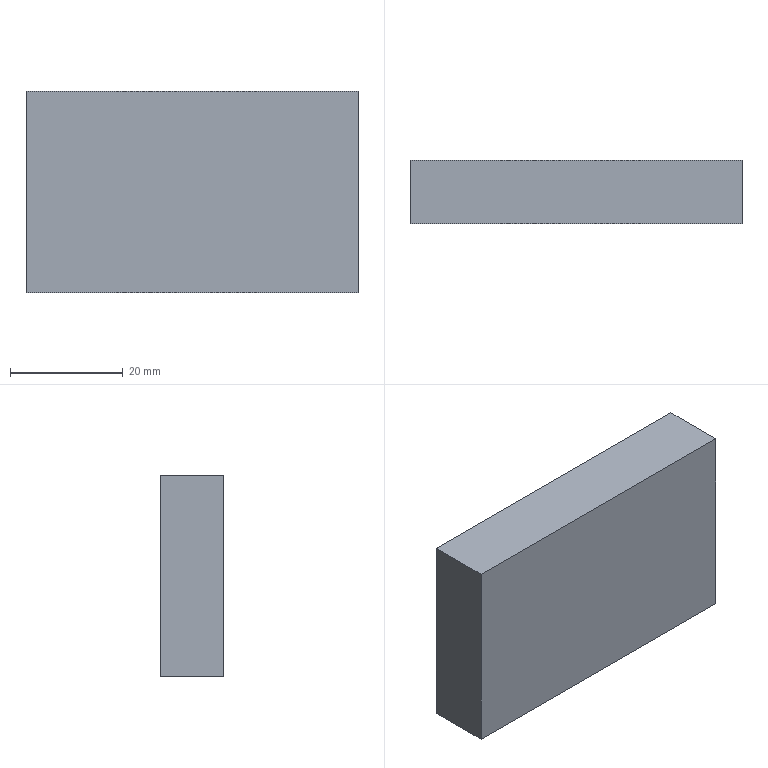Part | STEP file | 1 solid | 6 faces | box 58.8 x 11.27 x 35.77 mm | volume 23704 mm3 | plane 6
STEP:
#1=CARTESIAN_POINT('',(0.,0.,0.));
#2=DIRECTION('',(0.,0.,1.));
#3=DIRECTION('',(1.,0.,0.));
#4=AXIS2_PLACEMENT_3D('',#1,#2,#3);
#5=CARTESIAN_POINT('',(979.439,-73.009,179.647));
#6=VERTEX_POINT('',#5);
#7=CARTESIAN_POINT('',(920.639,-73.009,179.647));
#8=VERTEX_POINT('',#7);
#9=CARTESIAN_POINT('',(979.439,-73.009,179.647));
#10=DIRECTION('',(-1.,0.,0.));
#11=VECTOR('',#10,1.);
#12=LINE('',#9,#11);
#13=CARTESIAN_POINT('',(950.039,-67.374,179.647));
#14=DIRECTION('',(0.,0.,1.));
#15=DIRECTION('',(1.,0.,0.));
#16=AXIS2_PLACEMENT_3D('',#13,#14,#15);
#17=PLANE('',#16);
#18=CARTESIAN_POINT('',(29.4,-5.635));
#19=DIRECTION('',(-1.,0.));
#20=VECTOR('',#19,1.);
#21=LINE('',#18,#20);
#22=(GEOMETRIC_REPRESENTATION_CONTEXT(2)PARAMETRIC_REPRESENTATION_CONTEXT()REPRESENTATION_CONTEXT('',''));
#23=DEFINITIONAL_REPRESENTATION('',(#21),#22);
#24=PCURVE('',#17,#23);
#25=CARTESIAN_POINT('',(979.439,-73.009,143.877));
#26=DIRECTION('',(0.,1.,0.));
#27=DIRECTION('',(-1.,0.,0.));
#28=AXIS2_PLACEMENT_3D('',#25,#26,#27);
#29=PLANE('',#28);
#30=CARTESIAN_POINT('',(0.,35.77));
#31=DIRECTION('',(1.,0.));
#32=VECTOR('',#31,1.);
#33=LINE('',#30,#32);
#34=(GEOMETRIC_REPRESENTATION_CONTEXT(2)PARAMETRIC_REPRESENTATION_CONTEXT()REPRESENTATION_CONTEXT('',''));
#35=DEFINITIONAL_REPRESENTATION('',(#33),#34);
#36=PCURVE('',#29,#35);
#37=SURFACE_CURVE('',#12,(#24,#36),.PCURVE_S1.);
#38=EDGE_CURVE('',#6,#8,#37,.T.);
#39=ORIENTED_EDGE('',*,*,#38,.F.);
#40=CARTESIAN_POINT('',(979.439,-61.739,179.647));
#41=VERTEX_POINT('',#40);
#42=CARTESIAN_POINT('',(979.439,-73.009,179.647));
#43=DIRECTION('',(0.,1.,0.));
#44=VECTOR('',#43,1.);
#45=LINE('',#42,#44);
#46=CARTESIAN_POINT('',(29.4,-5.635));
#47=DIRECTION('',(0.,1.));
#48=VECTOR('',#47,1.);
#49=LINE('',#46,#48);
#50=(GEOMETRIC_REPRESENTATION_CONTEXT(2)PARAMETRIC_REPRESENTATION_CONTEXT()REPRESENTATION_CONTEXT('',''));
#51=DEFINITIONAL_REPRESENTATION('',(#49),#50);
#52=PCURVE('',#17,#51);
#53=CARTESIAN_POINT('',(979.439,-73.009,143.877));
#54=DIRECTION('',(1.,0.,0.));
#55=DIRECTION('',(0.,0.,-1.));
#56=AXIS2_PLACEMENT_3D('',#53,#54,#55);
#57=PLANE('',#56);
#58=CARTESIAN_POINT('',(-35.77,0.));
#59=DIRECTION('',(0.,1.));
#60=VECTOR('',#59,1.);
#61=LINE('',#58,#60);
#62=(GEOMETRIC_REPRESENTATION_CONTEXT(2)PARAMETRIC_REPRESENTATION_CONTEXT()REPRESENTATION_CONTEXT('',''));
#63=DEFINITIONAL_REPRESENTATION('',(#61),#62);
#64=PCURVE('',#57,#63);
#65=SURFACE_CURVE('',#45,(#52,#64),.PCURVE_S1.);
#66=EDGE_CURVE('',#6,#41,#65,.T.);
#67=ORIENTED_EDGE('',*,*,#66,.T.);
#68=CARTESIAN_POINT('',(920.639,-61.739,179.647));
#69=VERTEX_POINT('',#68);
#70=CARTESIAN_POINT('',(979.439,-61.739,179.647));
#71=DIRECTION('',(-1.,0.,0.));
#72=VECTOR('',#71,1.);
#73=LINE('',#70,#72);
#74=CARTESIAN_POINT('',(29.4,5.635));
#75=DIRECTION('',(-1.,0.));
#76=VECTOR('',#75,1.);
#77=LINE('',#74,#76);
#78=(GEOMETRIC_REPRESENTATION_CONTEXT(2)PARAMETRIC_REPRESENTATION_CONTEXT()REPRESENTATION_CONTEXT('',''));
#79=DEFINITIONAL_REPRESENTATION('',(#77),#78);
#80=PCURVE('',#17,#79);
#81=CARTESIAN_POINT('',(979.439,-61.739,143.877));
#82=DIRECTION('',(0.,1.,0.));
#83=DIRECTION('',(-1.,0.,0.));
#84=AXIS2_PLACEMENT_3D('',#81,#82,#83);
#85=PLANE('',#84);
#86=CARTESIAN_POINT('',(0.,35.77));
#87=DIRECTION('',(1.,0.));
#88=VECTOR('',#87,1.);
#89=LINE('',#86,#88);
#90=(GEOMETRIC_REPRESENTATION_CONTEXT(2)PARAMETRIC_REPRESENTATION_CONTEXT()REPRESENTATION_CONTEXT('',''));
#91=DEFINITIONAL_REPRESENTATION('',(#89),#90);
#92=PCURVE('',#85,#91);
#93=SURFACE_CURVE('',#73,(#80,#92),.PCURVE_S1.);
#94=EDGE_CURVE('',#41,#69,#93,.T.);
#95=ORIENTED_EDGE('',*,*,#94,.T.);
#96=CARTESIAN_POINT('',(920.639,-61.739,179.647));
#97=DIRECTION('',(0.,-1.,0.));
#98=VECTOR('',#97,1.);
#99=LINE('',#96,#98);
#100=CARTESIAN_POINT('',(-29.4,5.635));
#101=DIRECTION('',(0.,-1.));
#102=VECTOR('',#101,1.);
#103=LINE('',#100,#102);
#104=(GEOMETRIC_REPRESENTATION_CONTEXT(2)PARAMETRIC_REPRESENTATION_CONTEXT()REPRESENTATION_CONTEXT('',''));
#105=DEFINITIONAL_REPRESENTATION('',(#103),#104);
#106=PCURVE('',#17,#105);
#107=CARTESIAN_POINT('',(920.639,-61.739,143.877));
#108=DIRECTION('',(-1.,0.,0.));
#109=DIRECTION('',(0.,-1.,0.));
#110=AXIS2_PLACEMENT_3D('',#107,#108,#109);
#111=PLANE('',#110);
#112=CARTESIAN_POINT('',(0.,35.77));
#113=DIRECTION('',(1.,0.));
#114=VECTOR('',#113,1.);
#115=LINE('',#112,#114);
#116=(GEOMETRIC_REPRESENTATION_CONTEXT(2)PARAMETRIC_REPRESENTATION_CONTEXT()REPRESENTATION_CONTEXT('',''));
#117=DEFINITIONAL_REPRESENTATION('',(#115),#116);
#118=PCURVE('',#111,#117);
#119=SURFACE_CURVE('',#99,(#106,#118),.PCURVE_S1.);
#120=EDGE_CURVE('',#69,#8,#119,.T.);
#121=ORIENTED_EDGE('',*,*,#120,.T.);
#122=EDGE_LOOP('',(#39,#67,#95,#121));
#123=FACE_BOUND('',#122,.T.);
#124=ADVANCED_FACE('',(#123),#17,.T.);
#125=CARTESIAN_POINT('',(979.439,-73.009,143.877));
#126=VERTEX_POINT('',#125);
#127=CARTESIAN_POINT('',(920.639,-73.009,143.877));
#128=VERTEX_POINT('',#127);
#129=CARTESIAN_POINT('',(979.439,-73.009,143.877));
#130=DIRECTION('',(-1.,0.,0.));
#131=VECTOR('',#130,1.);
#132=LINE('',#129,#131);
#133=CARTESIAN_POINT('',(950.039,-67.374,143.877));
#134=DIRECTION('',(0.,0.,1.));
#135=DIRECTION('',(1.,0.,0.));
#136=AXIS2_PLACEMENT_3D('',#133,#134,#135);
#137=PLANE('',#136);
#138=CARTESIAN_POINT('',(29.4,-5.635));
#139=DIRECTION('',(-1.,0.));
#140=VECTOR('',#139,1.);
#141=LINE('',#138,#140);
#142=(GEOMETRIC_REPRESENTATION_CONTEXT(2)PARAMETRIC_REPRESENTATION_CONTEXT()REPRESENTATION_CONTEXT('',''));
#143=DEFINITIONAL_REPRESENTATION('',(#141),#142);
#144=PCURVE('',#137,#143);
#145=CARTESIAN_POINT('',(0.,0.));
#146=DIRECTION('',(1.,0.));
#147=VECTOR('',#146,1.);
#148=LINE('',#145,#147);
#149=(GEOMETRIC_REPRESENTATION_CONTEXT(2)PARAMETRIC_REPRESENTATION_CONTEXT()REPRESENTATION_CONTEXT('',''));
#150=DEFINITIONAL_REPRESENTATION('',(#148),#149);
#151=PCURVE('',#29,#150);
#152=SURFACE_CURVE('',#132,(#144,#151),.PCURVE_S1.);
#153=EDGE_CURVE('',#126,#128,#152,.T.);
#154=ORIENTED_EDGE('',*,*,#153,.T.);
#155=CARTESIAN_POINT('',(920.639,-61.739,143.877));
#156=VERTEX_POINT('',#155);
#157=CARTESIAN_POINT('',(920.639,-61.739,143.877));
#158=DIRECTION('',(0.,-1.,0.));
#159=VECTOR('',#158,1.);
#160=LINE('',#157,#159);
#161=CARTESIAN_POINT('',(-29.4,5.635));
#162=DIRECTION('',(0.,-1.));
#163=VECTOR('',#162,1.);
#164=LINE('',#161,#163);
#165=(GEOMETRIC_REPRESENTATION_CONTEXT(2)PARAMETRIC_REPRESENTATION_CONTEXT()REPRESENTATION_CONTEXT('',''));
#166=DEFINITIONAL_REPRESENTATION('',(#164),#165);
#167=PCURVE('',#137,#166);
#168=CARTESIAN_POINT('',(0.,0.));
#169=DIRECTION('',(1.,0.));
#170=VECTOR('',#169,1.);
#171=LINE('',#168,#170);
#172=(GEOMETRIC_REPRESENTATION_CONTEXT(2)PARAMETRIC_REPRESENTATION_CONTEXT()REPRESENTATION_CONTEXT('',''));
#173=DEFINITIONAL_REPRESENTATION('',(#171),#172);
#174=PCURVE('',#111,#173);
#175=SURFACE_CURVE('',#160,(#167,#174),.PCURVE_S1.);
#176=EDGE_CURVE('',#156,#128,#175,.T.);
#177=ORIENTED_EDGE('',*,*,#176,.F.);
#178=CARTESIAN_POINT('',(979.439,-61.739,143.877));
#179=VERTEX_POINT('',#178);
#180=CARTESIAN_POINT('',(979.439,-61.739,143.877));
#181=DIRECTION('',(-1.,0.,0.));
#182=VECTOR('',#181,1.);
#183=LINE('',#180,#182);
#184=CARTESIAN_POINT('',(29.4,5.635));
#185=DIRECTION('',(-1.,0.));
#186=VECTOR('',#185,1.);
#187=LINE('',#184,#186);
#188=(GEOMETRIC_REPRESENTATION_CONTEXT(2)PARAMETRIC_REPRESENTATION_CONTEXT()REPRESENTATION_CONTEXT('',''));
#189=DEFINITIONAL_REPRESENTATION('',(#187),#188);
#190=PCURVE('',#137,#189);
#191=CARTESIAN_POINT('',(0.,0.));
#192=DIRECTION('',(1.,0.));
#193=VECTOR('',#192,1.);
#194=LINE('',#191,#193);
#195=(GEOMETRIC_REPRESENTATION_CONTEXT(2)PARAMETRIC_REPRESENTATION_CONTEXT()REPRESENTATION_CONTEXT('',''));
#196=DEFINITIONAL_REPRESENTATION('',(#194),#195);
#197=PCURVE('',#85,#196);
#198=SURFACE_CURVE('',#183,(#190,#197),.PCURVE_S1.);
#199=EDGE_CURVE('',#179,#156,#198,.T.);
#200=ORIENTED_EDGE('',*,*,#199,.F.);
#201=CARTESIAN_POINT('',(979.439,-73.009,143.877));
#202=DIRECTION('',(0.,1.,0.));
#203=VECTOR('',#202,1.);
#204=LINE('',#201,#203);
#205=CARTESIAN_POINT('',(29.4,-5.635));
#206=DIRECTION('',(0.,1.));
#207=VECTOR('',#206,1.);
#208=LINE('',#205,#207);
#209=(GEOMETRIC_REPRESENTATION_CONTEXT(2)PARAMETRIC_REPRESENTATION_CONTEXT()REPRESENTATION_CONTEXT('',''));
#210=DEFINITIONAL_REPRESENTATION('',(#208),#209);
#211=PCURVE('',#137,#210);
#212=CARTESIAN_POINT('',(0.,0.));
#213=DIRECTION('',(0.,1.));
#214=VECTOR('',#213,1.);
#215=LINE('',#212,#214);
#216=(GEOMETRIC_REPRESENTATION_CONTEXT(2)PARAMETRIC_REPRESENTATION_CONTEXT()REPRESENTATION_CONTEXT('',''));
#217=DEFINITIONAL_REPRESENTATION('',(#215),#216);
#218=PCURVE('',#57,#217);
#219=SURFACE_CURVE('',#204,(#211,#218),.PCURVE_S1.);
#220=EDGE_CURVE('',#126,#179,#219,.T.);
#221=ORIENTED_EDGE('',*,*,#220,.F.);
#222=EDGE_LOOP('',(#154,#177,#200,#221));
#223=FACE_BOUND('',#222,.T.);
#224=ADVANCED_FACE('',(#223),#137,.F.);
#225=ORIENTED_EDGE('',*,*,#66,.F.);
#226=CARTESIAN_POINT('',(979.439,-73.009,143.877));
#227=DIRECTION('',(0.,0.,1.));
#228=VECTOR('',#227,1.);
#229=LINE('',#226,#228);
#230=CARTESIAN_POINT('',(0.,0.));
#231=DIRECTION('',(-1.,0.));
#232=VECTOR('',#231,1.);
#233=LINE('',#230,#232);
#234=(GEOMETRIC_REPRESENTATION_CONTEXT(2)PARAMETRIC_REPRESENTATION_CONTEXT()REPRESENTATION_CONTEXT('',''));
#235=DEFINITIONAL_REPRESENTATION('',(#233),#234);
#236=PCURVE('',#57,#235);
#237=CARTESIAN_POINT('',(0.,0.));
#238=DIRECTION('',(0.,1.));
#239=VECTOR('',#238,1.);
#240=LINE('',#237,#239);
#241=(GEOMETRIC_REPRESENTATION_CONTEXT(2)PARAMETRIC_REPRESENTATION_CONTEXT()REPRESENTATION_CONTEXT('',''));
#242=DEFINITIONAL_REPRESENTATION('',(#240),#241);
#243=PCURVE('',#29,#242);
#244=SURFACE_CURVE('',#229,(#236,#243),.PCURVE_S1.);
#245=EDGE_CURVE('',#126,#6,#244,.T.);
#246=ORIENTED_EDGE('',*,*,#245,.F.);
#247=ORIENTED_EDGE('',*,*,#220,.T.);
#248=CARTESIAN_POINT('',(979.439,-61.739,143.877));
#249=DIRECTION('',(0.,0.,1.));
#250=VECTOR('',#249,1.);
#251=LINE('',#248,#250);
#252=CARTESIAN_POINT('',(0.,11.27));
#253=DIRECTION('',(-1.,0.));
#254=VECTOR('',#253,1.);
#255=LINE('',#252,#254);
#256=(GEOMETRIC_REPRESENTATION_CONTEXT(2)PARAMETRIC_REPRESENTATION_CONTEXT()REPRESENTATION_CONTEXT('',''));
#257=DEFINITIONAL_REPRESENTATION('',(#255),#256);
#258=PCURVE('',#57,#257);
#259=CARTESIAN_POINT('',(0.,0.));
#260=DIRECTION('',(0.,1.));
#261=VECTOR('',#260,1.);
#262=LINE('',#259,#261);
#263=(GEOMETRIC_REPRESENTATION_CONTEXT(2)PARAMETRIC_REPRESENTATION_CONTEXT()REPRESENTATION_CONTEXT('',''));
#264=DEFINITIONAL_REPRESENTATION('',(#262),#263);
#265=PCURVE('',#85,#264);
#266=SURFACE_CURVE('',#251,(#258,#265),.PCURVE_S1.);
#267=EDGE_CURVE('',#179,#41,#266,.T.);
#268=ORIENTED_EDGE('',*,*,#267,.T.);
#269=EDGE_LOOP('',(#225,#246,#247,#268));
#270=FACE_BOUND('',#269,.T.);
#271=ADVANCED_FACE('',(#270),#57,.T.);
#272=ORIENTED_EDGE('',*,*,#94,.F.);
#273=ORIENTED_EDGE('',*,*,#267,.F.);
#274=ORIENTED_EDGE('',*,*,#199,.T.);
#275=CARTESIAN_POINT('',(920.639,-61.739,143.877));
#276=DIRECTION('',(0.,0.,1.));
#277=VECTOR('',#276,1.);
#278=LINE('',#275,#277);
#279=CARTESIAN_POINT('',(58.8,0.));
#280=DIRECTION('',(0.,1.));
#281=VECTOR('',#280,1.);
#282=LINE('',#279,#281);
#283=(GEOMETRIC_REPRESENTATION_CONTEXT(2)PARAMETRIC_REPRESENTATION_CONTEXT()REPRESENTATION_CONTEXT('',''));
#284=DEFINITIONAL_REPRESENTATION('',(#282),#283);
#285=PCURVE('',#85,#284);
#286=CARTESIAN_POINT('',(0.,0.));
#287=DIRECTION('',(0.,1.));
#288=VECTOR('',#287,1.);
#289=LINE('',#286,#288);
#290=(GEOMETRIC_REPRESENTATION_CONTEXT(2)PARAMETRIC_REPRESENTATION_CONTEXT()REPRESENTATION_CONTEXT('',''));
#291=DEFINITIONAL_REPRESENTATION('',(#289),#290);
#292=PCURVE('',#111,#291);
#293=SURFACE_CURVE('',#278,(#285,#292),.PCURVE_S1.);
#294=EDGE_CURVE('',#156,#69,#293,.T.);
#295=ORIENTED_EDGE('',*,*,#294,.T.);
#296=EDGE_LOOP('',(#272,#273,#274,#295));
#297=FACE_BOUND('',#296,.T.);
#298=ADVANCED_FACE('',(#297),#85,.T.);
#299=ORIENTED_EDGE('',*,*,#120,.F.);
#300=ORIENTED_EDGE('',*,*,#294,.F.);
#301=ORIENTED_EDGE('',*,*,#176,.T.);
#302=CARTESIAN_POINT('',(920.639,-73.009,143.877));
#303=DIRECTION('',(0.,0.,1.));
#304=VECTOR('',#303,1.);
#305=LINE('',#302,#304);
#306=CARTESIAN_POINT('',(11.27,0.));
#307=DIRECTION('',(0.,1.));
#308=VECTOR('',#307,1.);
#309=LINE('',#306,#308);
#310=(GEOMETRIC_REPRESENTATION_CONTEXT(2)PARAMETRIC_REPRESENTATION_CONTEXT()REPRESENTATION_CONTEXT('',''));
#311=DEFINITIONAL_REPRESENTATION('',(#309),#310);
#312=PCURVE('',#111,#311);
#313=CARTESIAN_POINT('',(58.8,0.));
#314=DIRECTION('',(0.,1.));
#315=VECTOR('',#314,1.);
#316=LINE('',#313,#315);
#317=(GEOMETRIC_REPRESENTATION_CONTEXT(2)PARAMETRIC_REPRESENTATION_CONTEXT()REPRESENTATION_CONTEXT('',''));
#318=DEFINITIONAL_REPRESENTATION('',(#316),#317);
#319=PCURVE('',#29,#318);
#320=SURFACE_CURVE('',#305,(#312,#319),.PCURVE_S1.);
#321=EDGE_CURVE('',#128,#8,#320,.T.);
#322=ORIENTED_EDGE('',*,*,#321,.T.);
#323=EDGE_LOOP('',(#299,#300,#301,#322));
#324=FACE_BOUND('',#323,.T.);
#325=ADVANCED_FACE('',(#324),#111,.T.);
#326=ORIENTED_EDGE('',*,*,#38,.T.);
#327=ORIENTED_EDGE('',*,*,#321,.F.);
#328=ORIENTED_EDGE('',*,*,#153,.F.);
#329=ORIENTED_EDGE('',*,*,#245,.T.);
#330=EDGE_LOOP('',(#326,#327,#328,#329));
#331=FACE_BOUND('',#330,.T.);
#332=ADVANCED_FACE('',(#331),#29,.F.);
#333=CLOSED_SHELL('',(#124,#224,#271,#298,#325,#332));
#334=MANIFOLD_SOLID_BREP('',#333);
#335=(LENGTH_UNIT()NAMED_UNIT(*)SI_UNIT(.MILLI.,.METRE.));
#336=UNCERTAINTY_MEASURE_WITH_UNIT(LENGTH_MEASURE(0.0000001),#335,'','');
#337=(NAMED_UNIT(*)PLANE_ANGLE_UNIT()SI_UNIT($,.RADIAN.));
#338=(NAMED_UNIT(*)SI_UNIT($,.STERADIAN.)SOLID_ANGLE_UNIT());
#339=(GEOMETRIC_REPRESENTATION_CONTEXT(3)GLOBAL_UNCERTAINTY_ASSIGNED_CONTEXT((#336))GLOBAL_UNIT_ASSIGNED_CONTEXT((#335,#337,#338))REPRESENTATION_CONTEXT('',''));
#340=ADVANCED_BREP_SHAPE_REPRESENTATION('',(#4,#334),#339);